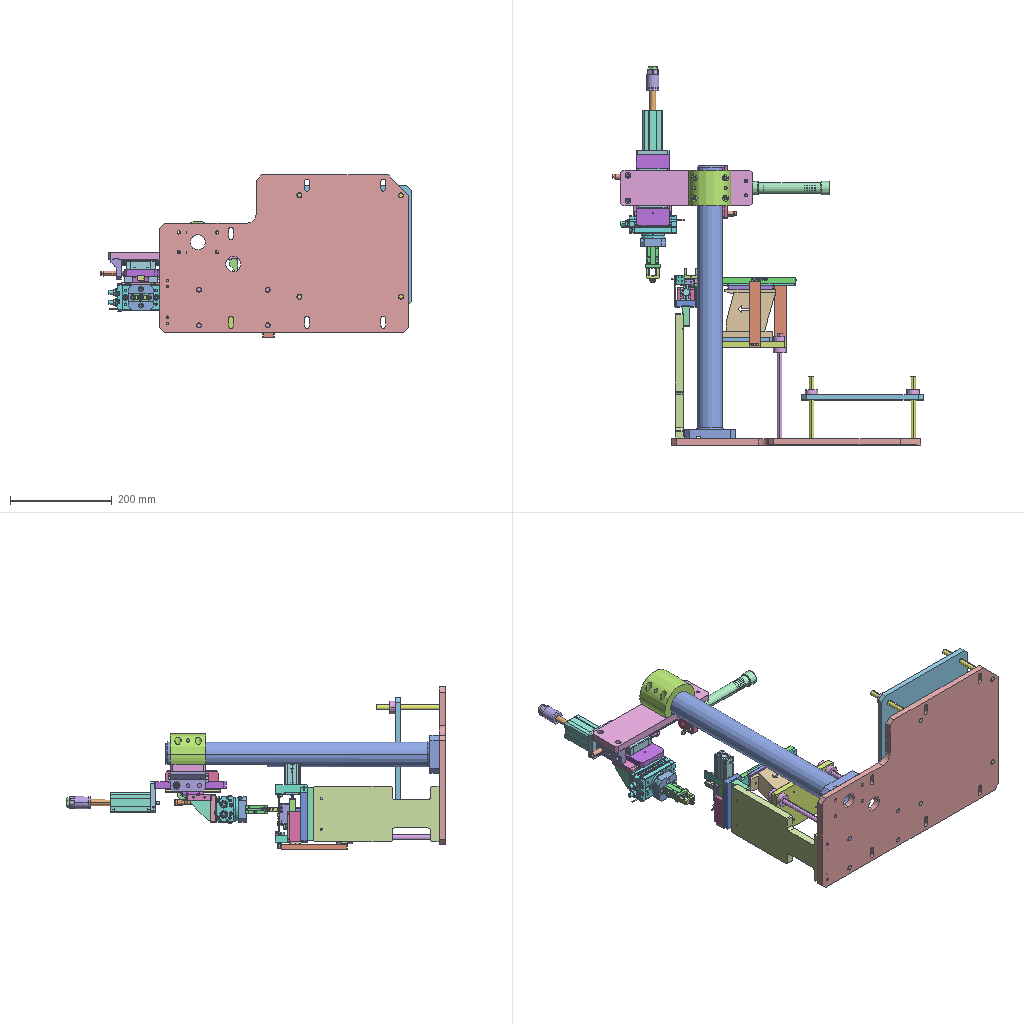Assembly | STEP file | 67 different items | 118 placed | box 611 x 745 x 319 mm
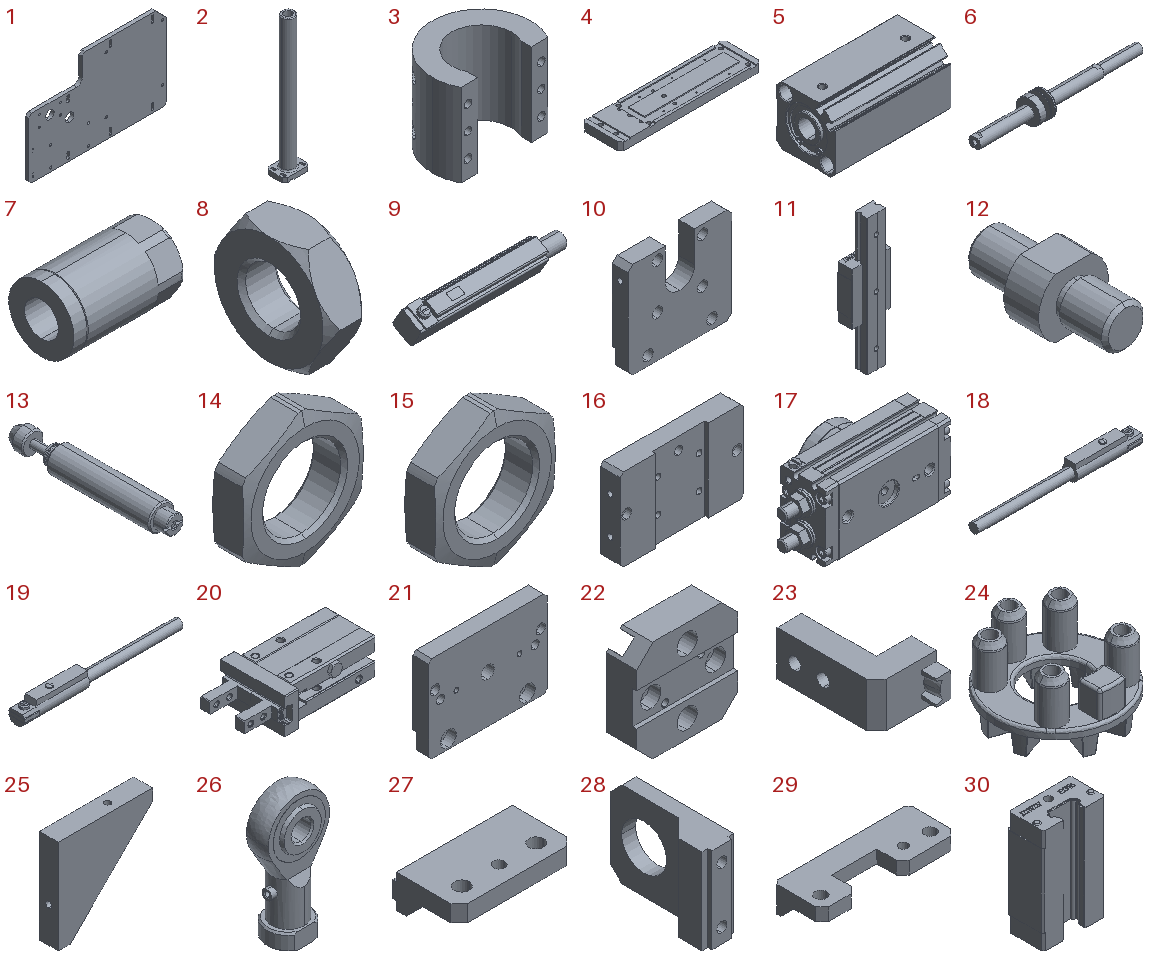Parts list (item | name | quantity | parent item | size | volume):
1 | PN_0035 | x1 | - | 490 x 12 x 310 mm | 1555006 mm3
2 | PN_0008 | x1 | in PN_0017 | 100 x 75 x 538 mm | 739254 mm3
3 | PN_0013 | x1 | in PN_0017 | 83 x 61 x 70 mm | 151269 mm3
4 | PN_0024 | x1 | in PN_0017 | 260 x 70 x 15 mm | 251185 mm3
5 | ACQJS-25x40-20-G-11 | x1 | in ACQJS-25x40-20-G-1 (00) | 79 x 40 x 40 mm | 79327 mm3
6 | ACQJS-25x40-20-G-12 | x1 | in ACQJS-25x40-20-G-1 (00) | 170.5 x 25 x 25 mm | 21717 mm3
7 | ACQJS-25x40-20-G-13 | x1 | in ACQJS-25x40-20-G-1 (00) | 41 x 24 x 24 mm | 13745 mm3
8 | ACQJS-25x40-20-G-14 | x1 | in ACQJS-25x40-20-G-1 (00) | 6 x 19.63 x 17 mm | 1118 mm3
9 | ACQJS-25x40-20-G-15 | x1 | in ACQJS-25x40-20-G-1 (00) | 30.5 x 5.877 x 6.057 mm | 552.742 mm3
10 | PN_0007 | x1 | in PN_0017 | 65 x 10 x 60 mm | 30379 mm3
11 | MGN15C | x1 | in PN_0017 | 32 x 16 x 110 mm | 27183 mm3
12 | PN_0037 | x1 | in PN_0017 | 10 x 20 x 8.5 mm | 768.323 mm3
13 | PA-1007-11 | x2 | in PA-1007-1 | 10 x 62 x 10 mm | 3798 mm3
14 | PA-1007-12 | x2 | in PA-1007-1 | 14 x 4 x 15.686 mm | 394.069 mm3
15 | PA-1007-13 | x2 | in PA-1007-1 | 14 x 4 x 15.686 mm | 394.069 mm3
16 | PN_0005 | x1 | in PN_0017 | 75 x 12 x 50 mm | 40001 mm3
17 | HRQ10-H-2-H-21 | x1 | in HRQ10-H-2-H-2 | 109.5 x 47 x 54.5 mm | 164782 mm3
18 | HRQ10-H-2-H-22 | x1 | in HRQ10-H-2-H-2 | 42 x 4 x 5.1 mm | 360.74 mm3
19 | HRQ10-H-2-H-23 | x1 | in HRQ10-H-2-H-2 | 42 x 4 x 5.1 mm | 360.74 mm3
20 | HFSZ10-CL-G-11 | x1 | in PN_0017 | 57 x 29 x 16.4 mm | 14404 mm3
21 | PN_0033 | x1 | in PN_0017 | 75 x 10 x 55 mm | 37025 mm3
22 | PN_0004 | x1 | in PN_0017 | 50 x 15 x 50 mm | 26390 mm3
23 | PN_0015 | x4 | in PN_0017 | 12.1 x 23 x 9 mm | 1039 mm3
24 | Product 3 | x20 | in PN_0017, PN_0041 | 11.8 x 11.8 x 6.802 mm | 181.296 mm3
25 | PN_0010 | x2 | in PN_0017 | 40 x 8 x 40 mm | 7824 mm3
26 | F-M06100U1 | x1 | in PN_0017 | - | 3624 mm3
27 | PN_0028 | x1 | in PN_0017 | 70 x 40 x 20 mm | 33206 mm3
28 | PN_0025 | x1 | in PN_0017 | 16 x 57 x 43 mm | 19963 mm3
29 | PN_0030 | x1 | in PN_0017 | 105 x 40 x 20 mm | 43466 mm3
30 | EGH15CA_BLOCK | x2 | in EGH15CA-160 | 34 x 19.5 x 57.8 mm | 30496 mm3
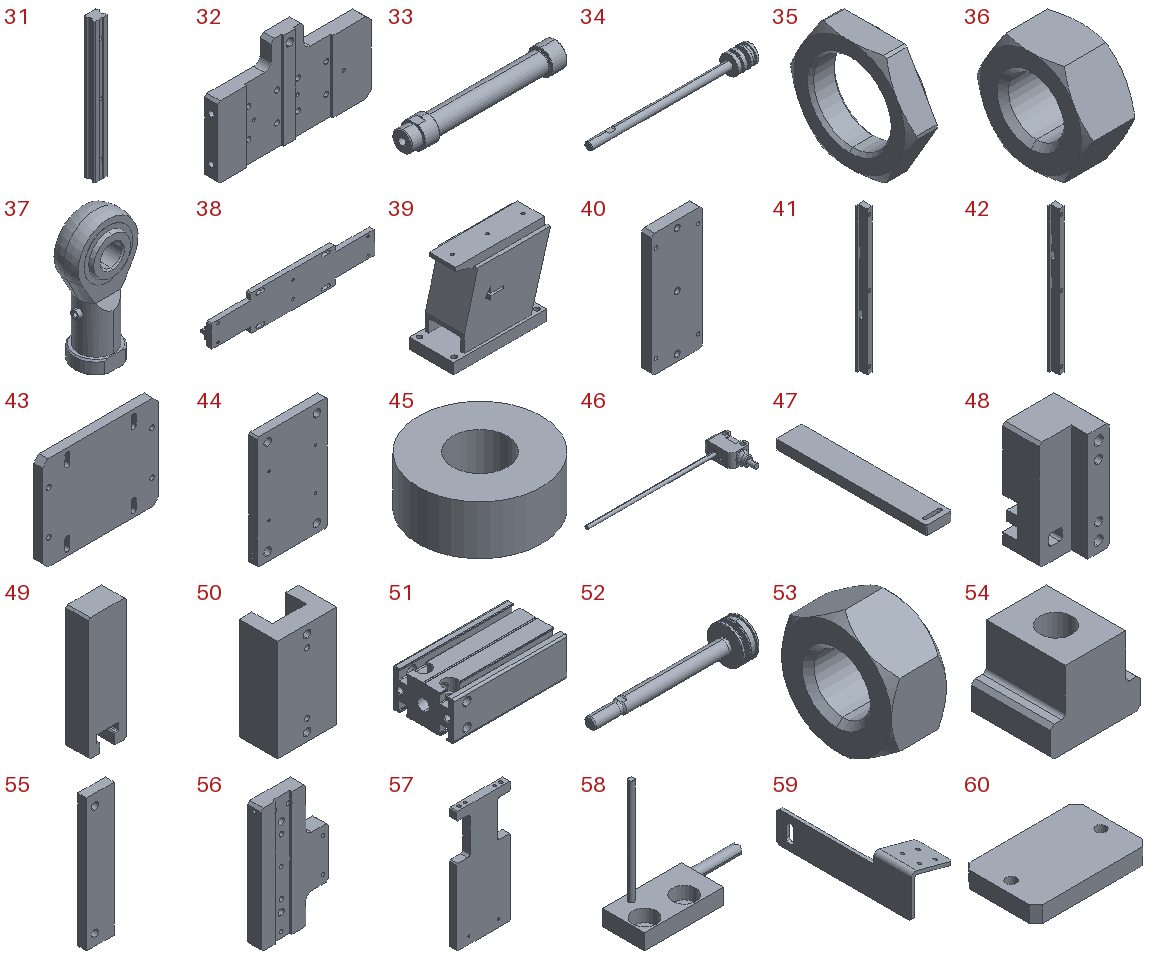31 | EG15_RAIL-160 | x2 | in EGH15CA-160 | 15 x 12.5 x 160 mm | 25521 mm3
32 | PN_0040 | x1 | in PN_0017 | 140 x 12 x 87.5 mm | 99789 mm3
33 | MA20x80-S-U-M-11 | x1 | in MA20x80-S-U-M-1 (0) | 168 x 27 x 27 mm | 32418 mm3
34 | MA20x80-S-U-M-12 | x1 | in MA20x80-S-U-M-1 (0) | 169 x 19.5 x 19.5 mm | 12396 mm3
35 | MA20x80-S-U-M-13 | x1 | in MA20x80-S-U-M-1 (0) | 7 x 33 x 29 mm | 2695 mm3
36 | MA20x80-S-U-M-14 | x1 | in MA20x80-S-U-M-1 (0) | 6 x 13.856 x 12 mm | 526.038 mm3
37 | F-M08125U | x1 | in PN_0017 | 24 x 14 x 48 mm | 6722 mm3
38 | PN_0018 | x1 | in PN_0041 | 175 x 10.7 x 37.5 mm | 32070 mm3
39 | 110 vibrator | x1 | in PN_0041 | 112 x 50 x 94 mm | 146734 mm3
40 | PN_0032 | x1 | in PN_0041 | 37.5 x 7.5 x 90 mm | 24273 mm3
41 | PN_0021 | x1 | in PN_0041 | 9 x 10.5 x 175 mm | 11358 mm3
42 | PN_0006 | x1 | in PN_0041 | 9 x 10.5 x 175 mm | 11358 mm3
43 | PN_0023 | x1 | in PN_0041 | 105 x 8 x 85 mm | 68896 mm3
44 | PN_0009 | x1 | in PN_0041 | 100 x 12 x 160 mm | 187185 mm3
45 | PN_0002 | x12 | in PN_0041 | 25 x 25 x 10 mm | 3958 mm3
46 | E3T-ST11 | x2 | in PN_0041 | 74.901 x 22.575 x 7 mm | 1025 mm3
47 | PN_0029 | x2 | in PN_0041 | 22.5 x 130.5 x 8 mm | 23047 mm3
48 | PN_0022 | x1 | - | 20 x 19.5 x 40 mm | 11103 mm3
49 | PN_0026 | x1 | - | 20 x 12 x 65 mm | 14321 mm3
50 | PN_0034 | x1 | - | 35 x 22.5 x 60 mm | 31897 mm3
51 | MD-16x20-S1 | x1 | in MD-16x20-S (0) | 60 x 32.2 x 20.2 mm | 24062 mm3
52 | MD-16x20-S2 | x1 | in MD-16x20-S (0) | 67 x 15.6 x 15.6 mm | 2736 mm3
53 | MD-16x20-S3 | x1 | in MD-16x20-S (0) | 4 x 8 x 9.238 mm | 163.482 mm3
54 | PN_0020 | x1 | - | 12 x 10.5 x 10 mm | 865.332 mm3
55 | PN_0027 | x2 | - | 12.5 x 4 x 60 mm | 2901 mm3
56 | PN_0001 | x1 | - | 60 x 12 x 110 mm | 56528 mm3
57 | PN_0012 | x1 | - | 110 x 15 x 247 mm | 337148 mm3
58 | Omron E32-T15ZR | x2 | - | 24.538 x 8 x 23 mm | 319.672 mm3
59 | PN_0014 | x2 | - | 19.319 x 62.5 x 19.394 mm | 1902 mm3
60 | PN_0031 | x1 | - | 35 x 22.5 x 5 mm | 3817 mm3
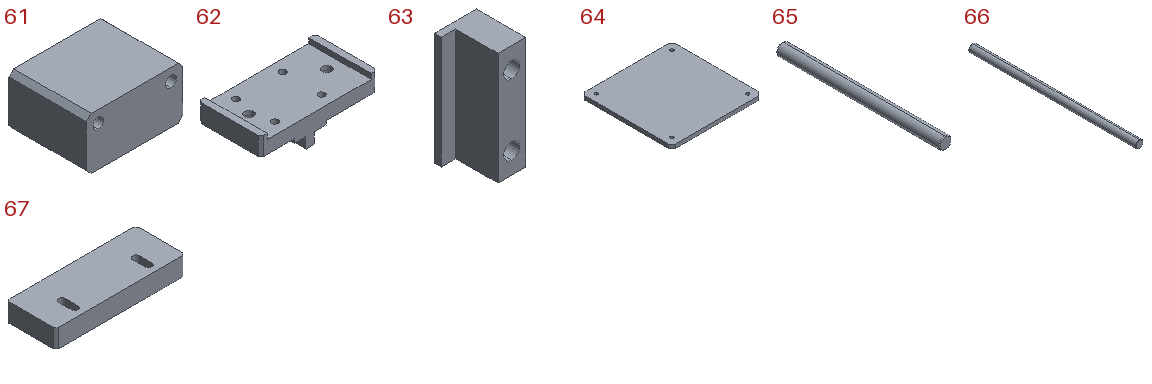61 | PN_0036 | x1 | - | 40 x 32 x 21.5 mm | 25854 mm3
62 | PN_0039 | x1 | - | 45 x 24 x 12.7 mm | 6100 mm3
63 | PN_0016 | x2 | - | 9 x 10.5 x 24 mm | 1408 mm3
64 | PN_0011 | x1 | - | 240 x 240 x 10 mm | 571730 mm3
65 | PN_0038 | x4 | - | 10 x 135 x 10 mm | 10595 mm3
66 | PN_0003 | x4 | - | 10 x 220 x 10 mm | 17271 mm3
67 | PN_0019 | x1 | - | 105 x 40 x 15 mm | 59951 mm3
Placements (level | parent | child | x y z in mm | rotation matrix by rows):
1 | subassembly 2 | PN_0035 | -41.882 -5.575 450.0 | 1 0 0 0 1 0 0 0 1
1 | subassembly 2 | PN_0017 | -209 -197.575 527.937 | 1 0 0 0 0 1 0 -1 0
2 | PN_0017 | PN_0008 | -2.882 7.937 213.0 | 1 0 0 0 1 0 0 0 1
2 | PN_0017 | PN_0013 | -2.882 7.937 698.0 | -1 0 0 0 -1 0 0 0 1
2 | PN_0017 | PN_0024 | 81.118 27.437 663.0 | -1 0 0 0 0 1 0 1 0
2 | PN_0017 | ACQJS-25x40-20-G-1 (00) | -115.132 102.907 771.5 | 0 0 1 0 -1 0 1 0 -0
3 | ACQJS-25x40-20-G-1 (00) | ACQJS-25x40-20-G-11 | -0.0 0.0 -0.0 | 1 0 0 0 1 0 0 0 1
3 | ACQJS-25x40-20-G-1 (00) | ACQJS-25x40-20-G-12 | -0.0 0.0 -0.0 | 1 0 0 0 1 0 0 0 1
3 | ACQJS-25x40-20-G-1 (00) | ACQJS-25x40-20-G-13 | -0.0 0.0 -0.0 | 1 0 0 0 1 0 0 0 1
3 | ACQJS-25x40-20-G-1 (00) | ACQJS-25x40-20-G-14 | -0.0 0.0 -0.0 | 1 0 0 0 1 0 0 0 1
3 | ACQJS-25x40-20-G-1 (00) | ACQJS-25x40-20-G-15 | -0.0 0.0 -0.0 | 1 0 0 0 1 0 0 0 1
2 | PN_0017 | PN_0007 | -115.132 92.407 771.5 | 1 0 0 0 0 1 0 -1 0
2 | PN_0017 | MGN15C | -115.132 72.407 688.5 | 1 0 0 0 1 0 0 0 1
2 | PN_0017 | PN_0037 | -115.132 102.907 766.5 | 0.9804 0 0.1969 -0.1969 0 0.9804 0 -1 0
2 | PN_0017 | PA-1007-1 | -193.882 69.437 720.5 | 0 1 0 -1 0 0 0 0 1
3 | PA-1007-1 | PA-1007-11 | 0.0 0.0 -0.0 | 1 0 0 0 1 0 0 0 1
3 | PA-1007-1 | PA-1007-12 | 0.0 0.0 -0.0 | 1 0 0 0 1 0 0 0 1
3 | PA-1007-1 | PA-1007-13 | 0.0 0.0 -0.0 | 1 0 0 0 1 0 0 0 1
2 | PN_0017 | PA-1007-1 | 50.118 69.437 648.0 | 0 -1 0 0.3818 0 0.9242 -0.9242 0 0.3818
3 | PA-1007-1 | PA-1007-11 | 0.0 0.0 -0.0 | 1 0 0 0 1 0 0 0 1
3 | PA-1007-1 | PA-1007-12 | 0.0 0.0 -0.0 | 1 0 0 0 1 0 0 0 1
3 | PA-1007-1 | PA-1007-13 | 0.0 0.0 -0.0 | 1 0 0 0 1 0 0 0 1
2 | PN_0017 | PN_0005 | -115.132 86.407 676.5 | 1 0 0 0 1 0 0 0 1
2 | PN_0017 | HRQ10-H-2-H-2 | -115.132 116.407 643.5 | 1 0 0 0 0 1 0 -1 -0
3 | HRQ10-H-2-H-2 | HRQ10-H-2-H-21 | 0.0 0.0 -0.0 | 1 0 0 0 1 0 0 0 1
3 | HRQ10-H-2-H-2 | HRQ10-H-2-H-22 | 0.0 0.0 -0.0 | 1 0 0 0 1 0 0 0 1
3 | HRQ10-H-2-H-2 | HRQ10-H-2-H-23 | 0.0 0.0 -0.0 | 1 0 0 0 1 0 0 0 1
2 | PN_0017 | HFSZ10-CL-G-11 | -115.132 116.407 585.5 | 0 1 0 0 0 1 1 0 -0
2 | PN_0017 | PN_0033 | -115.132 113.907 643.5 | -1 0 0 0 0 1 0 1 -0
2 | PN_0017 | PN_0004 | -115.132 116.407 583.5 | 1 0 0 0 0 -1 0 1 0
2 | PN_0017 | PN_0015 | -108.072 116.407 520.8 | -1 0 0 0 0 1 0 1 -0
2 | PN_0017 | PN_0015 | -122.192 116.407 520.8 | 1 0 0 0 0 -1 0 1 0
2 | PN_0017 | Product 3 | -115.142 116.407 517.7 | -1 0 0 0 1 0 0 0 -1
2 | PN_0017 | PN_0010 | -85.632 118.407 673.5 | 0 1 0 1 0 0 0 0 -1
2 | PN_0017 | PN_0010 | -144.632 118.407 673.5 | 0 -1 0 0 0 -1 1 0 0
2 | PN_0017 | PN_0015 | -47.192 116.407 520.8 | 1 0 0 0 0 -1 0 1 0
2 | PN_0017 | PN_0015 | -33.072 116.407 520.8 | -1 0 0 0 0 1 0 1 -0
2 | PN_0017 | F-M06100U1 | -115.132 102.907 724.0 | -1 0 0 0 1 0 0 0 -1
2 | PN_0017 | PN_0028 | -173.882 80.437 663.0 | 0 0 1 0 -1 0 1 0 -0
2 | PN_0017 | PN_0025 | 60.118 40.437 676.5 | 1 0 0 0 1 0 0 0 1
2 | PN_0017 | PN_0030 | 31.118 80.437 743.0 | 0 0 -1 0 -1 0 -1 0 0
2 | PN_0017 | EGH15CA-160 | -61.656 121.633 707.535 | 0 0 -1 0 1 0 1 0 0
3 | EGH15CA-160 | EGH15CA_BLOCK | 12.965 -57.226 33.576 | 1 0 0 0 1 0 0 0 1
3 | EGH15CA-160 | EG15_RAIL-160 | 12.965 -57.196 -10.274 | 1 0 0 0 1 0 0 0 1
2 | PN_0017 | PN_0040 | -82.632 62.407 763.5 | 0 0 1 0 1 0 -1 0 -0
2 | PN_0017 | EGH15CA-160 | -61.656 121.633 662.535 | 0 0 -1 0 1 0 1 0 0
3 | EGH15CA-160 | EGH15CA_BLOCK | 12.965 -57.226 33.576 | 1 0 0 0 1 0 0 0 1
3 | EGH15CA-160 | EG15_RAIL-160 | 12.965 -57.196 -10.274 | 1 0 0 0 1 0 0 0 1
2 | PN_0017 | MA20x80-S-U-M-1 (0) | 92.118 80.437 698.0 | 1 0 0 0 1 0 0 0 1
3 | MA20x80-S-U-M-1 (0) | MA20x80-S-U-M-11 | 0.0 -0.0 -0.0 | 1 0 0 0 1 0 0 0 1
3 | MA20x80-S-U-M-1 (0) | MA20x80-S-U-M-12 | 0.0 -0.0 -0.0 | 1 0 0 0 1 0 0 0 1
3 | MA20x80-S-U-M-1 (0) | MA20x80-S-U-M-13 | 0.0 -0.0 -0.0 | 1 0 0 0 1 0 0 0 1
3 | MA20x80-S-U-M-1 (0) | MA20x80-S-U-M-14 | 0.0 -0.0 -0.0 | 1 0 0 0 1 0 0 0 1
2 | PN_0017 | F-M08125U | -32.132 80.407 698.0 | 0 0 -1 0 1 0 1 0 0
1 | subassembly 2 | PN_0041 | -127.161 307.418 611.48 | -1 0 0 0 1 0 0 0 -1
2 | PN_0041 | PN_0018 | 4.261 1.007 220 | 1 0 0 0 1 0 0 0 1
2 | PN_0041 | Product 3 | 85.862 12.469 220.05 | 1 0 0 0 0 -1 0 1 0
2 | PN_0041 | Product 3 | 74.061 12.469 220.05 | 1 0 0 0 0 -1 0 1 0
2 | PN_0041 | Product 3 | 62.261 12.469 220.05 | 1 0 0 0 0 -1 0 1 0
2 | PN_0041 | Product 3 | 50.462 12.469 220.05 | 1 0 0 0 0 -1 0 1 0
2 | PN_0041 | Product 3 | 38.661 12.469 220.05 | 1 0 0 0 0 -1 0 1 0
2 | PN_0041 | Product 3 | 26.861 12.469 220.05 | 1 0 0 0 0 -1 0 1 0
2 | PN_0041 | Product 3 | 15.062 12.469 220.05 | 1 0 0 0 0 -1 0 1 0
2 | PN_0041 | Product 3 | 3.261 12.469 220.05 | 1 0 0 0 0 -1 0 1 0
2 | PN_0041 | Product 3 | -8.539 12.469 220.05 | 1 0 0 0 0 -1 0 1 0
2 | PN_0041 | Product 3 | -20.338 12.469 220.05 | 1 0 0 0 0 -1 0 1 0
2 | PN_0041 | Product 3 | -32.139 12.469 220.05 | 1 0 0 0 0 -1 0 1 0
2 | PN_0041 | Product 3 | -43.938 12.469 220.05 | 1 0 0 0 0 -1 0 1 0
2 | PN_0041 | Product 3 | -55.739 12.469 220.05 | 1 0 0 0 0 -1 0 1 0
2 | PN_0041 | Product 3 | -67.538 12.469 220.05 | 1 0 0 0 0 -1 0 1 0
2 | PN_0041 | Product 3 | -79.338 12.469 220.05 | 1 0 0 0 0 -1 0 1 0
2 | PN_0041 | 110 vibrator | 14.761 -94.493 220 | -1 0 0 0 0 1 0 1 0
2 | PN_0041 | PN_0032 | 4.261 -6.493 220 | 0 0 1 0 1 0 -1 0 0
2 | PN_0041 | PN_0021 | 4.261 6.007 212.5 | 0 0 1 0 1 0 -1 0 0
2 | PN_0041 | PN_0006 | 4.261 6.007 227.5 | 0 0 -1 0 1 0 1 0 0
2 | PN_0041 | PN_0023 | 14.761 -108.493 220 | 1 0 0 0 1 0 0 0 1
2 | PN_0041 | PN_0009 | 14.761 -120.493 220 | 0 0 1 0 1 0 -1 0 0
2 | PN_0041 | PN_0002 | -52.739 -98.493 255 | 0.8372 -0.5469 0 0 0 -1 0.5469 0.8372 0
2 | PN_0041 | PN_0002 | -52.739 -130.493 255 | 1 0 0 0 0 1 0 -1 -0
2 | PN_0041 | PN_0002 | -52.739 -130.493 185 | 1 0 0 0 0 1 0 -1 -0
2 | PN_0041 | PN_0002 | 82.261 -130.493 255 | 1 0 0 0 0 1 0 -1 -0
2 | PN_0041 | PN_0002 | 82.261 -130.493 185 | 1 0 0 0 0 1 0 -1 -0
2 | PN_0041 | PN_0002 | -52.739 -98.493 185 | 0.8372 -0.5469 0 0 0 -1 0.5469 0.8372 0
2 | PN_0041 | PN_0002 | 82.261 -98.493 255 | 0.8372 -0.5469 0 0 0 -1 0.5469 0.8372 0
2 | PN_0041 | PN_0002 | 82.261 -98.493 185 | 0.8372 -0.5469 0 0 0 -1 0.5469 0.8372 0
2 | PN_0041 | E3T-ST11 | -195.334 10.007 151.203 | -0.4226 0.9063 0 0 0 1 0.9063 0.4226 0
2 | PN_0041 | E3T-ST11 | -188.55 17.007 136.655 | 0.4226 0.9063 0 0 0 -1 -0.9063 0.4226 -0
2 | PN_0041 | PN_0029 | -53.989 -55.243 270 | 1 0 0 0 1 0 0 0 1
2 | PN_0041 | PN_0029 | -3.627 -55.243 162 | 1 0 0 0 1 0 0 0 1
1 | subassembly 2 | PN_0022 | -253.022 306.925 402.53 | -1 0 0 0 1 0 0 0 -1
1 | subassembly 2 | Product 3 | -249.122 319.887 411.53 | -1 0 0 0 0 -1 0 -1 -0
1 | subassembly 2 | PN_0026 | -259.022 288.925 400.03 | -1 0 0 0 1 0 0 0 -1
1 | subassembly 2 | PN_0034 | -259.022 278.425 377.53 | 1 0 0 0 1 0 0 0 1
1 | subassembly 2 | MD-16x20-S (0) | -259.022 295.425 441.53 | 0 -0.01037 0.9999 0 -0.9999 -0.01037 1 0 -0
2 | MD-16x20-S (0) | MD-16x20-S1 | -0.0 -0.0 -0.0 | 1 0 0 0 1 0 0 0 1
2 | MD-16x20-S (0) | MD-16x20-S2 | -0.0 -0.0 -0.0 | 1 0 0 0 1 0 0 0 1
2 | MD-16x20-S (0) | MD-16x20-S3 | -0.0 -0.0 -0.0 | 1 0 0 0 1 0 0 0 1
1 | subassembly 2 | PN_0020 | -259.022 290.175 428.03 | 1 0 0 0 1 0 0 0 1
1 | subassembly 2 | PN_0027 | -247.772 300.925 377.53 | -1 0 0 0 1 0 0 0 -1
1 | subassembly 2 | PN_0027 | -270.272 300.925 377.53 | 1 0 0 0 1 0 0 0 1
1 | subassembly 2 | PN_0001 | -259.022 266.425 402.53 | 1 0 0 0 1 0 0 0 1
1 | subassembly 2 | PN_0012 | -279.522 129.925 402.53 | 0 1 0 0 0 -1 -1 0 -0
1 | subassembly 2 | Product 3 | -249.122 319.887 391.53 | -1 0 0 0 0 -1 0 -1 -0
1 | subassembly 2 | Omron E32-T15ZR | -242.352 319.925 364.945 | -0.9659 0 -0.2588 0 -1 0 -0.2588 0 0.9659
1 | subassembly 2 | PN_0014 | -237.522 328.925 366.239 | -1 0 0 0 -1 0 0 0 1
1 | subassembly 2 | PN_0014 | -280.522 328.925 439.784 | 1 0 0 0 -1 0 0 0 -1
1 | subassembly 2 | Omron E32-T15ZR | -263.619 322.925 444.313 | -0.9659 0 0.2588 0 1 0 -0.2588 0 -0.9659
1 | subassembly 2 | PN_0031 | -259.022 289.675 342.53 | 1 0 0 0 1 0 0 0 1
1 | subassembly 2 | PN_0036 | -240.522 292.425 395.03 | 0 0 1 0 1 0 -1 0 0
1 | subassembly 2 | PN_0039 | -231.022 319.125 395.03 | 0 -1 0 0 0 -1 1 0 -0
1 | subassembly 2 | PN_0016 | -231.022 313.425 383.98 | 0 0 1 0 1 0 -1 0 0
1 | subassembly 2 | PN_0016 | -231.022 313.425 398.98 | 0 0 -1 0 1 0 1 0 -0
1 | subassembly 2 | Product 3 | -237.322 319.887 391.53 | -1 0 0 0 0 -1 0 -1 -0
1 | subassembly 2 | Product 3 | -225.522 319.887 391.53 | -1 0 0 0 0 -1 0 -1 -0
1 | subassembly 2 | PN_0011 | 88.118 93.125 512.5 | 1 0 0 0 0 -1 0 1 0
1 | subassembly 2 | PN_0038 | 188.118 -5.575 412.5 | 1 0 0 0 1 0 0 0 1
1 | subassembly 2 | PN_0002 | 188.118 103.125 412.5 | 1 0 0 0 0 -1 0 1 0
1 | subassembly 2 | PN_0003 | -74.382 -5.575 356.5 | 1 0 0 0 1 0 0 0 1
1 | subassembly 2 | PN_0003 | -209.382 -5.575 426.5 | 1 0 0 0 1 0 0 0 1
1 | subassembly 2 | PN_0003 | -74.382 -5.575 426.5 | 1 0 0 0 1 0 0 0 1
1 | subassembly 2 | PN_0003 | -209.382 -5.575 356.5 | 1 0 0 0 1 0 0 0 1
1 | subassembly 2 | PN_0038 | -11.882 -5.575 412.5 | 1 0 0 0 1 0 0 0 1
1 | subassembly 2 | PN_0038 | 188.118 -5.575 612.5 | 1 0 0 0 1 0 0 0 1
1 | subassembly 2 | PN_0038 | -11.882 -5.575 612.5 | 1 0 0 0 1 0 0 0 1
1 | subassembly 2 | PN_0002 | -11.882 103.125 412.5 | 1 0 0 0 0 -1 0 1 0
1 | subassembly 2 | PN_0002 | 188.118 103.125 612.5 | 1 0 0 0 0 -1 0 1 0
1 | subassembly 2 | PN_0002 | -11.882 103.125 612.5 | 1 0 0 0 0 -1 0 1 0
1 | subassembly 2 | PN_0019 | -266.522 248.425 402.53 | 0 0 1 0 1 0 -1 0 0